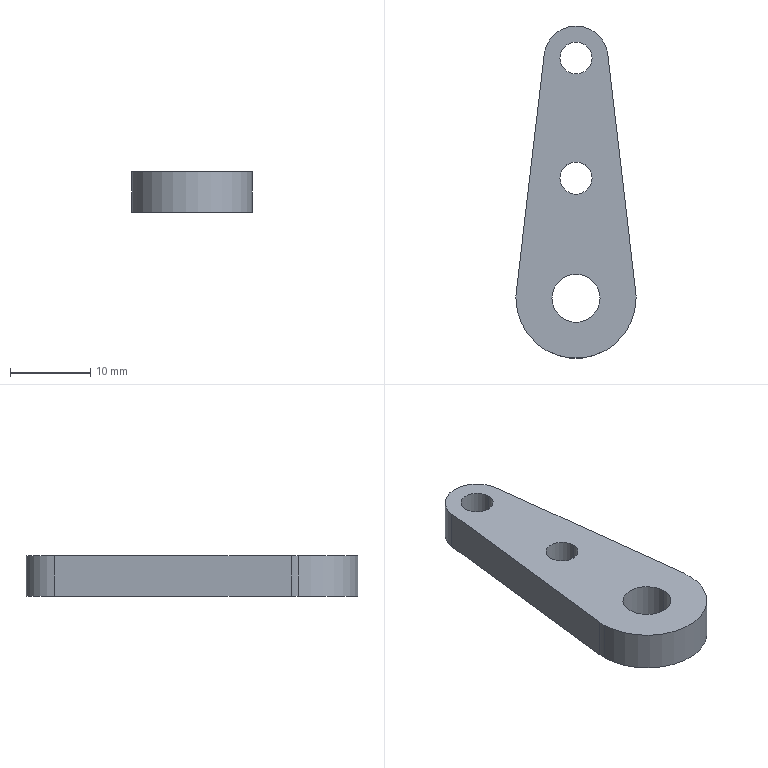Part | SolidWorks | features Extrusion 1, ICE 1 | 1 solid | 14 faces | box 15 x 41.5 x 5 mm | volume 2037 mm3 | cylinder 10 | plane 4 | commonest cylinder face diameters 4 x4 15 x3 6 x2 8 x1
STEP:
#1=CARTESIAN_POINT('',(-2.,15.,0.));
#2=VERTEX_POINT('',#1);
#3=CARTESIAN_POINT('',(2.,15.,0.));
#4=VERTEX_POINT('',#3);
#5=CARTESIAN_POINT('',(0.,15.,0.));
#6=DIRECTION('',(0.,0.,1.));
#7=DIRECTION('',(1.,0.,0.));
#8=AXIS2_PLACEMENT_3D('',#5,#6,#7);
#9=CIRCLE('',#8,2.);
#10=EDGE_CURVE('',#2,#4,#9,.T.);
#11=ORIENTED_EDGE('',*,*,#10,.F.);
#12=CARTESIAN_POINT('',(-2.,15.,5.));
#13=VERTEX_POINT('',#12);
#14=CARTESIAN_POINT('',(-2.,15.,0.));
#15=DIRECTION('',(0.,0.,1.));
#16=VECTOR('',#15,1000.);
#17=LINE('',#14,#16);
#18=EDGE_CURVE('',#2,#13,#17,.T.);
#19=ORIENTED_EDGE('',*,*,#18,.T.);
#20=CARTESIAN_POINT('',(2.,15.,5.));
#21=VERTEX_POINT('',#20);
#22=CARTESIAN_POINT('',(0.,15.,5.));
#23=DIRECTION('',(0.,0.,1.));
#24=DIRECTION('',(1.,0.,0.));
#25=AXIS2_PLACEMENT_3D('',#22,#23,#24);
#26=CIRCLE('',#25,2.);
#27=EDGE_CURVE('',#13,#21,#26,.T.);
#28=ORIENTED_EDGE('',*,*,#27,.T.);
#29=CARTESIAN_POINT('',(2.,15.,0.));
#30=DIRECTION('',(0.,0.,1.));
#31=VECTOR('',#30,1000.);
#32=LINE('',#29,#31);
#33=EDGE_CURVE('',#4,#21,#32,.T.);
#34=ORIENTED_EDGE('',*,*,#33,.F.);
#35=EDGE_LOOP('',(#11,#19,#28,#34));
#36=FACE_OUTER_BOUND('',#35,.T.);
#37=CARTESIAN_POINT('',(0.,15.,0.));
#38=DIRECTION('',(0.,0.,1.));
#39=DIRECTION('',(1.,0.,0.));
#40=AXIS2_PLACEMENT_3D('',#37,#38,#39);
#41=CYLINDRICAL_SURFACE('',#40,2.);
#42=ADVANCED_FACE('',(#36),#41,.F.);
#43=CARTESIAN_POINT('',(-3.,0.,5.));
#44=VERTEX_POINT('',#43);
#45=CARTESIAN_POINT('',(3.,0.,5.));
#46=VERTEX_POINT('',#45);
#47=CARTESIAN_POINT('',(0.,0.,5.));
#48=DIRECTION('',(0.,0.,1.));
#49=DIRECTION('',(1.,0.,0.));
#50=AXIS2_PLACEMENT_3D('',#47,#48,#49);
#51=CIRCLE('',#50,3.);
#52=EDGE_CURVE('',#44,#46,#51,.T.);
#53=ORIENTED_EDGE('',*,*,#52,.T.);
#54=CARTESIAN_POINT('',(3.,0.,0.));
#55=VERTEX_POINT('',#54);
#56=CARTESIAN_POINT('',(3.,0.,5.));
#57=DIRECTION('',(0.,0.,-1.));
#58=VECTOR('',#57,1000.);
#59=LINE('',#56,#58);
#60=EDGE_CURVE('',#46,#55,#59,.T.);
#61=ORIENTED_EDGE('',*,*,#60,.T.);
#62=CARTESIAN_POINT('',(-3.,0.,0.));
#63=VERTEX_POINT('',#62);
#64=CARTESIAN_POINT('',(0.,0.,0.));
#65=DIRECTION('',(0.,0.,1.));
#66=DIRECTION('',(1.,0.,0.));
#67=AXIS2_PLACEMENT_3D('',#64,#65,#66);
#68=CIRCLE('',#67,3.);
#69=EDGE_CURVE('',#63,#55,#68,.T.);
#70=ORIENTED_EDGE('',*,*,#69,.F.);
#71=CARTESIAN_POINT('',(-3.,0.,5.));
#72=DIRECTION('',(0.,0.,-1.));
#73=VECTOR('',#72,1000.);
#74=LINE('',#71,#73);
#75=EDGE_CURVE('',#44,#63,#74,.T.);
#76=ORIENTED_EDGE('',*,*,#75,.F.);
#77=EDGE_LOOP('',(#53,#61,#70,#76));
#78=FACE_OUTER_BOUND('',#77,.T.);
#79=CARTESIAN_POINT('',(0.,0.,5.));
#80=DIRECTION('',(0.,0.,-1.));
#81=DIRECTION('',(-1.,0.,0.));
#82=AXIS2_PLACEMENT_3D('',#79,#80,#81);
#83=CYLINDRICAL_SURFACE('',#82,3.);
#84=ADVANCED_FACE('',(#78),#83,.F.);
#85=CARTESIAN_POINT('',(-2.,30.,5.));
#86=VERTEX_POINT('',#85);
#87=CARTESIAN_POINT('',(2.,30.,5.));
#88=VERTEX_POINT('',#87);
#89=CARTESIAN_POINT('',(0.,30.,5.));
#90=DIRECTION('',(0.,0.,1.));
#91=DIRECTION('',(1.,0.,0.));
#92=AXIS2_PLACEMENT_3D('',#89,#90,#91);
#93=CIRCLE('',#92,2.);
#94=EDGE_CURVE('',#86,#88,#93,.T.);
#95=ORIENTED_EDGE('',*,*,#94,.T.);
#96=CARTESIAN_POINT('',(2.,30.,0.));
#97=VERTEX_POINT('',#96);
#98=CARTESIAN_POINT('',(2.,30.,5.));
#99=DIRECTION('',(0.,0.,-1.));
#100=VECTOR('',#99,1000.);
#101=LINE('',#98,#100);
#102=EDGE_CURVE('',#88,#97,#101,.T.);
#103=ORIENTED_EDGE('',*,*,#102,.T.);
#104=CARTESIAN_POINT('',(-2.,30.,0.));
#105=VERTEX_POINT('',#104);
#106=CARTESIAN_POINT('',(0.,30.,0.));
#107=DIRECTION('',(0.,0.,1.));
#108=DIRECTION('',(1.,0.,0.));
#109=AXIS2_PLACEMENT_3D('',#106,#107,#108);
#110=CIRCLE('',#109,2.);
#111=EDGE_CURVE('',#105,#97,#110,.T.);
#112=ORIENTED_EDGE('',*,*,#111,.F.);
#113=CARTESIAN_POINT('',(-2.,30.,5.));
#114=DIRECTION('',(0.,0.,-1.));
#115=VECTOR('',#114,1000.);
#116=LINE('',#113,#115);
#117=EDGE_CURVE('',#86,#105,#116,.T.);
#118=ORIENTED_EDGE('',*,*,#117,.F.);
#119=EDGE_LOOP('',(#95,#103,#112,#118));
#120=FACE_OUTER_BOUND('',#119,.T.);
#121=CARTESIAN_POINT('',(0.,30.,5.));
#122=DIRECTION('',(0.,0.,-1.));
#123=DIRECTION('',(-1.,0.,0.));
#124=AXIS2_PLACEMENT_3D('',#121,#122,#123);
#125=CYLINDRICAL_SURFACE('',#124,2.);
#126=ADVANCED_FACE('',(#120),#125,.F.);
#127=CARTESIAN_POINT('',(7.5,0.,5.));
#128=VERTEX_POINT('',#127);
#129=CARTESIAN_POINT('',(7.449,0.875,5.));
#130=VERTEX_POINT('',#129);
#131=CARTESIAN_POINT('',(0.,0.,5.));
#132=DIRECTION('',(0.,0.,1.));
#133=DIRECTION('',(1.,0.,0.));
#134=AXIS2_PLACEMENT_3D('',#131,#132,#133);
#135=CIRCLE('',#134,7.5);
#136=EDGE_CURVE('',#128,#130,#135,.T.);
#137=ORIENTED_EDGE('',*,*,#136,.F.);
#138=CARTESIAN_POINT('',(7.5,0.,0.));
#139=VERTEX_POINT('',#138);
#140=CARTESIAN_POINT('',(7.5,0.,5.));
#141=DIRECTION('',(0.,0.,-1.));
#142=VECTOR('',#141,1000.);
#143=LINE('',#140,#142);
#144=EDGE_CURVE('',#128,#139,#143,.T.);
#145=ORIENTED_EDGE('',*,*,#144,.T.);
#146=CARTESIAN_POINT('',(7.449,0.875,0.));
#147=VERTEX_POINT('',#146);
#148=CARTESIAN_POINT('',(0.,0.,0.));
#149=DIRECTION('',(0.,0.,1.));
#150=DIRECTION('',(1.,0.,0.));
#151=AXIS2_PLACEMENT_3D('',#148,#149,#150);
#152=CIRCLE('',#151,7.5);
#153=EDGE_CURVE('',#139,#147,#152,.T.);
#154=ORIENTED_EDGE('',*,*,#153,.T.);
#155=CARTESIAN_POINT('',(7.449,0.875,5.));
#156=DIRECTION('',(0.,0.,-1.));
#157=VECTOR('',#156,1000.);
#158=LINE('',#155,#157);
#159=EDGE_CURVE('',#130,#147,#158,.T.);
#160=ORIENTED_EDGE('',*,*,#159,.F.);
#161=EDGE_LOOP('',(#137,#145,#154,#160));
#162=FACE_OUTER_BOUND('',#161,.T.);
#163=CARTESIAN_POINT('',(0.,0.,5.));
#164=DIRECTION('',(0.,0.,-1.));
#165=DIRECTION('',(-1.,0.,0.));
#166=AXIS2_PLACEMENT_3D('',#163,#164,#165);
#167=CYLINDRICAL_SURFACE('',#166,7.5);
#168=ADVANCED_FACE('',(#162),#167,.T.);
#169=ORIENTED_EDGE('',*,*,#144,.F.);
#170=CARTESIAN_POINT('',(-7.5,0.,5.));
#171=VERTEX_POINT('',#170);
#172=CARTESIAN_POINT('',(0.,0.,5.));
#173=DIRECTION('',(0.,0.,1.));
#174=DIRECTION('',(1.,0.,0.));
#175=AXIS2_PLACEMENT_3D('',#172,#173,#174);
#176=CIRCLE('',#175,7.5);
#177=EDGE_CURVE('',#171,#128,#176,.T.);
#178=ORIENTED_EDGE('',*,*,#177,.F.);
#179=CARTESIAN_POINT('',(-7.5,0.,0.));
#180=VERTEX_POINT('',#179);
#181=CARTESIAN_POINT('',(-7.5,0.,5.));
#182=DIRECTION('',(0.,0.,-1.));
#183=VECTOR('',#182,1000.);
#184=LINE('',#181,#183);
#185=EDGE_CURVE('',#171,#180,#184,.T.);
#186=ORIENTED_EDGE('',*,*,#185,.T.);
#187=CARTESIAN_POINT('',(0.,0.,0.));
#188=DIRECTION('',(0.,0.,1.));
#189=DIRECTION('',(1.,0.,0.));
#190=AXIS2_PLACEMENT_3D('',#187,#188,#189);
#191=CIRCLE('',#190,7.5);
#192=EDGE_CURVE('',#180,#139,#191,.T.);
#193=ORIENTED_EDGE('',*,*,#192,.T.);
#194=EDGE_LOOP('',(#169,#178,#186,#193));
#195=FACE_OUTER_BOUND('',#194,.T.);
#196=CARTESIAN_POINT('',(0.,0.,5.));
#197=DIRECTION('',(0.,0.,-1.));
#198=DIRECTION('',(-1.,0.,0.));
#199=AXIS2_PLACEMENT_3D('',#196,#197,#198);
#200=CYLINDRICAL_SURFACE('',#199,7.5);
#201=ADVANCED_FACE('',(#195),#200,.T.);
#202=CARTESIAN_POINT('',(0.,15.,5.));
#203=DIRECTION('',(0.,0.,1.));
#204=DIRECTION('',(1.,0.,0.));
#205=AXIS2_PLACEMENT_3D('',#202,#203,#204);
#206=CIRCLE('',#205,2.);
#207=EDGE_CURVE('',#21,#13,#206,.T.);
#208=ORIENTED_EDGE('',*,*,#207,.F.);
#209=ORIENTED_EDGE('',*,*,#27,.F.);
#210=EDGE_LOOP('',(#208,#209));
#211=FACE_BOUND('',#210,.T.);
#212=ORIENTED_EDGE('',*,*,#94,.F.);
#213=CARTESIAN_POINT('',(0.,30.,5.));
#214=DIRECTION('',(0.,0.,1.));
#215=DIRECTION('',(1.,0.,0.));
#216=AXIS2_PLACEMENT_3D('',#213,#214,#215);
#217=CIRCLE('',#216,2.);
#218=EDGE_CURVE('',#88,#86,#217,.T.);
#219=ORIENTED_EDGE('',*,*,#218,.F.);
#220=EDGE_LOOP('',(#212,#219));
#221=FACE_BOUND('',#220,.T.);
#222=CARTESIAN_POINT('',(3.973,30.467,5.));
#223=VERTEX_POINT('',#222);
#224=CARTESIAN_POINT('',(-3.973,30.467,5.));
#225=VERTEX_POINT('',#224);
#226=CARTESIAN_POINT('',(0.,30.,5.));
#227=DIRECTION('',(0.,0.,1.));
#228=DIRECTION('',(1.,0.,0.));
#229=AXIS2_PLACEMENT_3D('',#226,#227,#228);
#230=CIRCLE('',#229,4.);
#231=EDGE_CURVE('',#223,#225,#230,.T.);
#232=ORIENTED_EDGE('',*,*,#231,.T.);
#233=CARTESIAN_POINT('',(-7.449,0.875,5.));
#234=VERTEX_POINT('',#233);
#235=CARTESIAN_POINT('',(-3.973,30.467,5.));
#236=DIRECTION('',(-0.1167,-0.9932,0.));
#237=VECTOR('',#236,1000.);
#238=LINE('',#235,#237);
#239=EDGE_CURVE('',#225,#234,#238,.T.);
#240=ORIENTED_EDGE('',*,*,#239,.T.);
#241=CARTESIAN_POINT('',(0.,0.,5.));
#242=DIRECTION('',(0.,0.,1.));
#243=DIRECTION('',(1.,0.,0.));
#244=AXIS2_PLACEMENT_3D('',#241,#242,#243);
#245=CIRCLE('',#244,7.5);
#246=EDGE_CURVE('',#234,#171,#245,.T.);
#247=ORIENTED_EDGE('',*,*,#246,.T.);
#248=ORIENTED_EDGE('',*,*,#177,.T.);
#249=ORIENTED_EDGE('',*,*,#136,.T.);
#250=CARTESIAN_POINT('',(3.973,30.467,5.));
#251=DIRECTION('',(-0.1167,0.9932,0.));
#252=VECTOR('',#251,1000.);
#253=LINE('',#250,#252);
#254=EDGE_CURVE('',#130,#223,#253,.T.);
#255=ORIENTED_EDGE('',*,*,#254,.T.);
#256=EDGE_LOOP('',(#232,#240,#247,#248,#249,#255));
#257=FACE_OUTER_BOUND('',#256,.T.);
#258=ORIENTED_EDGE('',*,*,#52,.F.);
#259=CARTESIAN_POINT('',(0.,0.,5.));
#260=DIRECTION('',(0.,0.,1.));
#261=DIRECTION('',(1.,0.,0.));
#262=AXIS2_PLACEMENT_3D('',#259,#260,#261);
#263=CIRCLE('',#262,3.);
#264=EDGE_CURVE('',#46,#44,#263,.T.);
#265=ORIENTED_EDGE('',*,*,#264,.F.);
#266=EDGE_LOOP('',(#258,#265));
#267=FACE_BOUND('',#266,.T.);
#268=CARTESIAN_POINT('',(0.,30.,5.));
#269=DIRECTION('',(0.,0.,1.));
#270=DIRECTION('',(1.,0.,0.));
#271=AXIS2_PLACEMENT_3D('',#268,#269,#270);
#272=PLANE('',#271);
#273=ADVANCED_FACE('',(#211,#221,#257,#267),#272,.T.);
#274=CARTESIAN_POINT('',(0.,15.,0.));
#275=DIRECTION('',(0.,0.,1.));
#276=DIRECTION('',(1.,0.,0.));
#277=AXIS2_PLACEMENT_3D('',#274,#275,#276);
#278=CIRCLE('',#277,2.);
#279=EDGE_CURVE('',#4,#2,#278,.T.);
#280=ORIENTED_EDGE('',*,*,#279,.T.);
#281=ORIENTED_EDGE('',*,*,#10,.T.);
#282=EDGE_LOOP('',(#280,#281));
#283=FACE_BOUND('',#282,.T.);
#284=CARTESIAN_POINT('',(3.973,30.467,0.));
#285=VERTEX_POINT('',#284);
#286=CARTESIAN_POINT('',(-3.973,30.467,0.));
#287=VERTEX_POINT('',#286);
#288=CARTESIAN_POINT('',(0.,30.,0.));
#289=DIRECTION('',(0.,0.,1.));
#290=DIRECTION('',(1.,0.,0.));
#291=AXIS2_PLACEMENT_3D('',#288,#289,#290);
#292=CIRCLE('',#291,4.);
#293=EDGE_CURVE('',#285,#287,#292,.T.);
#294=ORIENTED_EDGE('',*,*,#293,.F.);
#295=CARTESIAN_POINT('',(3.973,30.467,0.));
#296=DIRECTION('',(-0.1167,0.9932,0.));
#297=VECTOR('',#296,1000.);
#298=LINE('',#295,#297);
#299=EDGE_CURVE('',#147,#285,#298,.T.);
#300=ORIENTED_EDGE('',*,*,#299,.F.);
#301=ORIENTED_EDGE('',*,*,#153,.F.);
#302=ORIENTED_EDGE('',*,*,#192,.F.);
#303=CARTESIAN_POINT('',(-7.449,0.875,0.));
#304=VERTEX_POINT('',#303);
#305=CARTESIAN_POINT('',(0.,0.,0.));
#306=DIRECTION('',(0.,0.,1.));
#307=DIRECTION('',(1.,0.,0.));
#308=AXIS2_PLACEMENT_3D('',#305,#306,#307);
#309=CIRCLE('',#308,7.5);
#310=EDGE_CURVE('',#304,#180,#309,.T.);
#311=ORIENTED_EDGE('',*,*,#310,.F.);
#312=CARTESIAN_POINT('',(-3.973,30.467,0.));
#313=DIRECTION('',(-0.1167,-0.9932,0.));
#314=VECTOR('',#313,1000.);
#315=LINE('',#312,#314);
#316=EDGE_CURVE('',#287,#304,#315,.T.);
#317=ORIENTED_EDGE('',*,*,#316,.F.);
#318=EDGE_LOOP('',(#294,#300,#301,#302,#311,#317));
#319=FACE_OUTER_BOUND('',#318,.T.);
#320=ORIENTED_EDGE('',*,*,#111,.T.);
#321=CARTESIAN_POINT('',(0.,30.,0.));
#322=DIRECTION('',(0.,0.,1.));
#323=DIRECTION('',(1.,0.,0.));
#324=AXIS2_PLACEMENT_3D('',#321,#322,#323);
#325=CIRCLE('',#324,2.);
#326=EDGE_CURVE('',#97,#105,#325,.T.);
#327=ORIENTED_EDGE('',*,*,#326,.T.);
#328=EDGE_LOOP('',(#320,#327));
#329=FACE_BOUND('',#328,.T.);
#330=ORIENTED_EDGE('',*,*,#69,.T.);
#331=CARTESIAN_POINT('',(0.,0.,0.));
#332=DIRECTION('',(0.,0.,1.));
#333=DIRECTION('',(1.,0.,0.));
#334=AXIS2_PLACEMENT_3D('',#331,#332,#333);
#335=CIRCLE('',#334,3.);
#336=EDGE_CURVE('',#55,#63,#335,.T.);
#337=ORIENTED_EDGE('',*,*,#336,.T.);
#338=EDGE_LOOP('',(#330,#337));
#339=FACE_BOUND('',#338,.T.);
#340=CARTESIAN_POINT('',(0.,30.,0.));
#341=DIRECTION('',(0.,0.,1.));
#342=DIRECTION('',(1.,0.,0.));
#343=AXIS2_PLACEMENT_3D('',#340,#341,#342);
#344=PLANE('',#343);
#345=ADVANCED_FACE('',(#283,#319,#329,#339),#344,.F.);
#346=ORIENTED_EDGE('',*,*,#293,.T.);
#347=CARTESIAN_POINT('',(-3.973,30.467,5.));
#348=DIRECTION('',(0.,0.,-1.));
#349=VECTOR('',#348,1000.);
#350=LINE('',#347,#349);
#351=EDGE_CURVE('',#225,#287,#350,.T.);
#352=ORIENTED_EDGE('',*,*,#351,.F.);
#353=ORIENTED_EDGE('',*,*,#231,.F.);
#354=CARTESIAN_POINT('',(3.973,30.467,5.));
#355=DIRECTION('',(0.,0.,-1.));
#356=VECTOR('',#355,1000.);
#357=LINE('',#354,#356);
#358=EDGE_CURVE('',#223,#285,#357,.T.);
#359=ORIENTED_EDGE('',*,*,#358,.T.);
#360=EDGE_LOOP('',(#346,#352,#353,#359));
#361=FACE_OUTER_BOUND('',#360,.T.);
#362=CARTESIAN_POINT('',(0.,30.,5.));
#363=DIRECTION('',(0.,0.,-1.));
#364=DIRECTION('',(-1.,0.,0.));
#365=AXIS2_PLACEMENT_3D('',#362,#363,#364);
#366=CYLINDRICAL_SURFACE('',#365,4.);
#367=ADVANCED_FACE('',(#361),#366,.T.);
#368=ORIENTED_EDGE('',*,*,#316,.T.);
#369=CARTESIAN_POINT('',(-7.449,0.875,5.));
#370=DIRECTION('',(0.,0.,-1.));
#371=VECTOR('',#370,1000.);
#372=LINE('',#369,#371);
#373=EDGE_CURVE('',#234,#304,#372,.T.);
#374=ORIENTED_EDGE('',*,*,#373,.F.);
#375=ORIENTED_EDGE('',*,*,#239,.F.);
#376=ORIENTED_EDGE('',*,*,#351,.T.);
#377=EDGE_LOOP('',(#368,#374,#375,#376));
#378=FACE_OUTER_BOUND('',#377,.T.);
#379=CARTESIAN_POINT('',(-3.973,30.467,5.));
#380=DIRECTION('',(0.9932,-0.1167,0.));
#381=DIRECTION('',(0.1167,0.9932,0.));
#382=AXIS2_PLACEMENT_3D('',#379,#380,#381);
#383=PLANE('',#382);
#384=ADVANCED_FACE('',(#378),#383,.F.);
#385=ORIENTED_EDGE('',*,*,#185,.F.);
#386=ORIENTED_EDGE('',*,*,#246,.F.);
#387=ORIENTED_EDGE('',*,*,#373,.T.);
#388=ORIENTED_EDGE('',*,*,#310,.T.);
#389=EDGE_LOOP('',(#385,#386,#387,#388));
#390=FACE_OUTER_BOUND('',#389,.T.);
#391=CARTESIAN_POINT('',(0.,0.,5.));
#392=DIRECTION('',(0.,0.,-1.));
#393=DIRECTION('',(-1.,0.,0.));
#394=AXIS2_PLACEMENT_3D('',#391,#392,#393);
#395=CYLINDRICAL_SURFACE('',#394,7.5);
#396=ADVANCED_FACE('',(#390),#395,.T.);
#397=ORIENTED_EDGE('',*,*,#299,.T.);
#398=ORIENTED_EDGE('',*,*,#358,.F.);
#399=ORIENTED_EDGE('',*,*,#254,.F.);
#400=ORIENTED_EDGE('',*,*,#159,.T.);
#401=EDGE_LOOP('',(#397,#398,#399,#400));
#402=FACE_OUTER_BOUND('',#401,.T.);
#403=CARTESIAN_POINT('',(3.973,30.467,5.));
#404=DIRECTION('',(-0.9932,-0.1167,0.));
#405=DIRECTION('',(0.1167,-0.9932,0.));
#406=AXIS2_PLACEMENT_3D('',#403,#404,#405);
#407=PLANE('',#406);
#408=ADVANCED_FACE('',(#402),#407,.F.);
#409=ORIENTED_EDGE('',*,*,#102,.F.);
#410=ORIENTED_EDGE('',*,*,#218,.T.);
#411=ORIENTED_EDGE('',*,*,#117,.T.);
#412=ORIENTED_EDGE('',*,*,#326,.F.);
#413=EDGE_LOOP('',(#409,#410,#411,#412));
#414=FACE_OUTER_BOUND('',#413,.T.);
#415=CARTESIAN_POINT('',(0.,30.,5.));
#416=DIRECTION('',(0.,0.,-1.));
#417=DIRECTION('',(-1.,0.,0.));
#418=AXIS2_PLACEMENT_3D('',#415,#416,#417);
#419=CYLINDRICAL_SURFACE('',#418,2.);
#420=ADVANCED_FACE('',(#414),#419,.F.);
#421=ORIENTED_EDGE('',*,*,#60,.F.);
#422=ORIENTED_EDGE('',*,*,#264,.T.);
#423=ORIENTED_EDGE('',*,*,#75,.T.);
#424=ORIENTED_EDGE('',*,*,#336,.F.);
#425=EDGE_LOOP('',(#421,#422,#423,#424));
#426=FACE_OUTER_BOUND('',#425,.T.);
#427=CARTESIAN_POINT('',(0.,0.,5.));
#428=DIRECTION('',(0.,0.,-1.));
#429=DIRECTION('',(-1.,0.,0.));
#430=AXIS2_PLACEMENT_3D('',#427,#428,#429);
#431=CYLINDRICAL_SURFACE('',#430,3.);
#432=ADVANCED_FACE('',(#426),#431,.F.);
#433=ORIENTED_EDGE('',*,*,#18,.F.);
#434=ORIENTED_EDGE('',*,*,#279,.F.);
#435=ORIENTED_EDGE('',*,*,#33,.T.);
#436=ORIENTED_EDGE('',*,*,#207,.T.);
#437=EDGE_LOOP('',(#433,#434,#435,#436));
#438=FACE_OUTER_BOUND('',#437,.T.);
#439=CARTESIAN_POINT('',(0.,15.,0.));
#440=DIRECTION('',(0.,0.,1.));
#441=DIRECTION('',(1.,0.,0.));
#442=AXIS2_PLACEMENT_3D('',#439,#440,#441);
#443=CYLINDRICAL_SURFACE('',#442,2.);
#444=ADVANCED_FACE('',(#438),#443,.F.);
#445=CLOSED_SHELL('',(#42,#84,#126,#168,#201,#273,#345,#367,#384,#396,#408,#420,#432,#444));
#446=MANIFOLD_SOLID_BREP('',#445);
#447=CARTESIAN_POINT('',(0.,0.,0.));
#448=DIRECTION('',(0.,0.,1.));
#449=DIRECTION('',(1.,0.,0.));
#450=AXIS2_PLACEMENT_3D('',#447,#448,#449);
#451=(LENGTH_UNIT()NAMED_UNIT(*)SI_UNIT(.MILLI.,.METRE.));
#452=UNCERTAINTY_MEASURE_WITH_UNIT(LENGTH_MEASURE(0.00001),#451,'','');
#453=(NAMED_UNIT(*)PLANE_ANGLE_UNIT()SI_UNIT($,.RADIAN.));
#454=(NAMED_UNIT(*)SI_UNIT($,.STERADIAN.)SOLID_ANGLE_UNIT());
#455=(GEOMETRIC_REPRESENTATION_CONTEXT(3)GLOBAL_UNCERTAINTY_ASSIGNED_CONTEXT((#452))GLOBAL_UNIT_ASSIGNED_CONTEXT((#451,#453,#454))REPRESENTATION_CONTEXT('',''));
#456=ADVANCED_BREP_SHAPE_REPRESENTATION('',(#446,#450),#455);